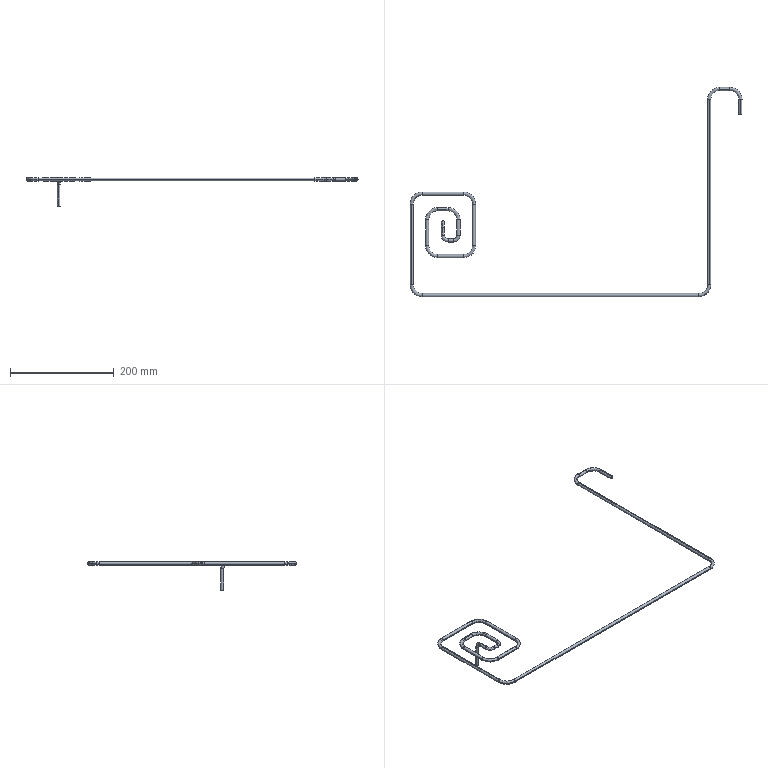Part | STEP file | copper tube 19_default_machined_ | 1 solid | 110 faces | box 638.85 x 402.7 x 54.675 mm | volume 25549 mm3 | cylinder 56 | spline 52 | plane 2 | commonest cylinder face diameters 4.75 x28 6.35 x28